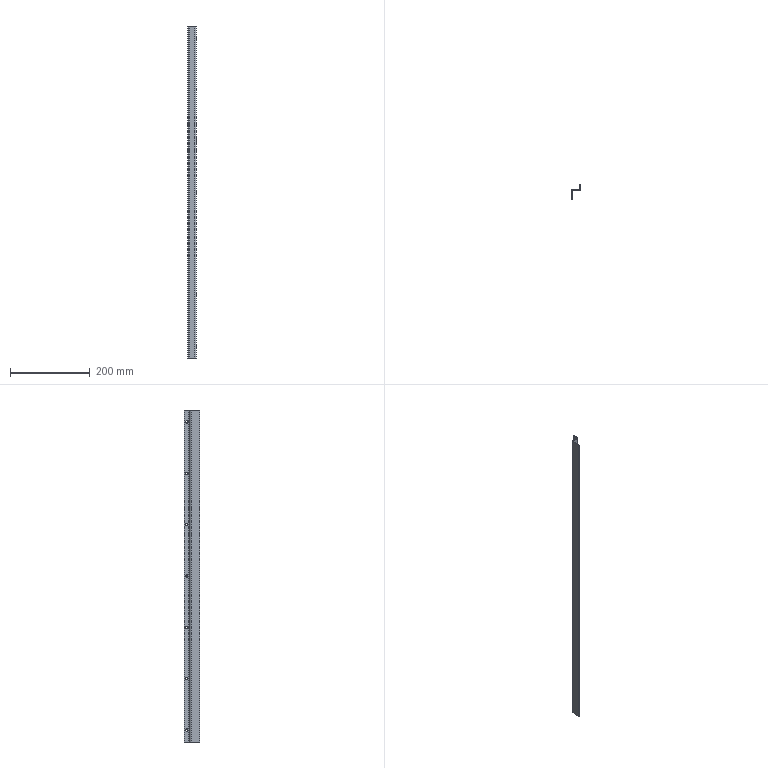Part | NX | features solid 2 | 1 solid | 28 faces | box 22 x 38 x 835 mm | volume 92164 mm3 | cylinder 18 | plane 10 | commonest cylinder face diameters 6 x14 4 x2 8 x2
STEP:
#1=CARTESIAN_POINT('',(1106.,-69.,920.));
#2=VERTEX_POINT('',#1);
#3=CARTESIAN_POINT('',(1108.,-69.,920.));
#4=VERTEX_POINT('',#3);
#5=CARTESIAN_POINT('',(1942.154,-69.,920.));
#6=DIRECTION('',(-1.,0.,0.));
#7=VECTOR('',#6,1000.);
#8=LINE('',#5,#7);
#9=EDGE_CURVE('',#2,#4,#8,.F.);
#10=ORIENTED_EDGE('',*,*,#9,.T.);
#11=CARTESIAN_POINT('',(1108.,-63.,920.));
#12=VERTEX_POINT('',#11);
#13=CARTESIAN_POINT('',(1108.,-66.,920.));
#14=DIRECTION('',(-1.,0.,0.));
#15=DIRECTION('',(0.,1.,0.));
#16=AXIS2_PLACEMENT_3D('',#13,#14,#15);
#17=CIRCLE('',#16,3.);
#18=EDGE_CURVE('',#12,#4,#17,.T.);
#19=ORIENTED_EDGE('',*,*,#18,.F.);
#20=CARTESIAN_POINT('',(1106.,-63.,920.));
#21=VERTEX_POINT('',#20);
#22=CARTESIAN_POINT('',(1942.154,-63.,920.));
#23=DIRECTION('',(-1.,0.,0.));
#24=VECTOR('',#23,1000.);
#25=LINE('',#22,#24);
#26=EDGE_CURVE('',#12,#21,#25,.T.);
#27=ORIENTED_EDGE('',*,*,#26,.T.);
#28=CARTESIAN_POINT('',(1106.,-66.,920.));
#29=DIRECTION('',(-1.,0.,0.));
#30=DIRECTION('',(0.,0.,1.));
#31=AXIS2_PLACEMENT_3D('',#28,#29,#30);
#32=CIRCLE('',#31,3.);
#33=EDGE_CURVE('',#21,#2,#32,.T.);
#34=ORIENTED_EDGE('',*,*,#33,.T.);
#35=EDGE_LOOP('',(#10,#19,#27,#34));
#36=FACE_BOUND('',#35,.T.);
#37=CARTESIAN_POINT('',(1942.154,-66.,920.));
#38=DIRECTION('',(-1.,0.,0.));
#39=DIRECTION('',(0.,1.,0.));
#40=AXIS2_PLACEMENT_3D('',#37,#38,#39);
#41=CYLINDRICAL_SURFACE('',#40,3.);
#42=ADVANCED_FACE('',(#36),#41,.F.);
#43=CARTESIAN_POINT('',(1108.,-69.,790.833));
#44=VERTEX_POINT('',#43);
#45=CARTESIAN_POINT('',(1106.,-69.,790.833));
#46=VERTEX_POINT('',#45);
#47=CARTESIAN_POINT('',(1942.154,-69.,790.833));
#48=DIRECTION('',(-1.,0.,0.));
#49=VECTOR('',#48,1000.);
#50=LINE('',#47,#49);
#51=EDGE_CURVE('',#44,#46,#50,.T.);
#52=ORIENTED_EDGE('',*,*,#51,.F.);
#53=CARTESIAN_POINT('',(1108.,-63.,790.833));
#54=VERTEX_POINT('',#53);
#55=CARTESIAN_POINT('',(1108.,-66.,790.833));
#56=DIRECTION('',(-1.,0.,0.));
#57=DIRECTION('',(0.,1.,0.));
#58=AXIS2_PLACEMENT_3D('',#55,#56,#57);
#59=CIRCLE('',#58,3.);
#60=EDGE_CURVE('',#54,#44,#59,.T.);
#61=ORIENTED_EDGE('',*,*,#60,.F.);
#62=CARTESIAN_POINT('',(1106.,-63.,790.833));
#63=VERTEX_POINT('',#62);
#64=CARTESIAN_POINT('',(1942.154,-63.,790.833));
#65=DIRECTION('',(-1.,0.,0.));
#66=VECTOR('',#65,1000.);
#67=LINE('',#64,#66);
#68=EDGE_CURVE('',#63,#54,#67,.F.);
#69=ORIENTED_EDGE('',*,*,#68,.F.);
#70=CARTESIAN_POINT('',(1106.,-66.,790.833));
#71=DIRECTION('',(-1.,0.,0.));
#72=DIRECTION('',(0.,0.,1.));
#73=AXIS2_PLACEMENT_3D('',#70,#71,#72);
#74=CIRCLE('',#73,3.);
#75=EDGE_CURVE('',#63,#46,#74,.T.);
#76=ORIENTED_EDGE('',*,*,#75,.T.);
#77=EDGE_LOOP('',(#52,#61,#69,#76));
#78=FACE_BOUND('',#77,.T.);
#79=CARTESIAN_POINT('',(1942.154,-66.,790.833));
#80=DIRECTION('',(-1.,0.,0.));
#81=DIRECTION('',(0.,1.,0.));
#82=AXIS2_PLACEMENT_3D('',#79,#80,#81);
#83=CYLINDRICAL_SURFACE('',#82,3.);
#84=ADVANCED_FACE('',(#78),#83,.F.);
#85=CARTESIAN_POINT('',(1108.,-69.,661.667));
#86=VERTEX_POINT('',#85);
#87=CARTESIAN_POINT('',(1106.,-69.,661.667));
#88=VERTEX_POINT('',#87);
#89=CARTESIAN_POINT('',(1942.154,-69.,661.667));
#90=DIRECTION('',(-1.,0.,0.));
#91=VECTOR('',#90,1000.);
#92=LINE('',#89,#91);
#93=EDGE_CURVE('',#86,#88,#92,.T.);
#94=ORIENTED_EDGE('',*,*,#93,.F.);
#95=CARTESIAN_POINT('',(1108.,-63.,661.667));
#96=VERTEX_POINT('',#95);
#97=CARTESIAN_POINT('',(1108.,-66.,661.667));
#98=DIRECTION('',(-1.,0.,0.));
#99=DIRECTION('',(0.,1.,0.));
#100=AXIS2_PLACEMENT_3D('',#97,#98,#99);
#101=CIRCLE('',#100,3.);
#102=EDGE_CURVE('',#96,#86,#101,.T.);
#103=ORIENTED_EDGE('',*,*,#102,.F.);
#104=CARTESIAN_POINT('',(1106.,-63.,661.667));
#105=VERTEX_POINT('',#104);
#106=CARTESIAN_POINT('',(1942.154,-63.,661.667));
#107=DIRECTION('',(-1.,0.,0.));
#108=VECTOR('',#107,1000.);
#109=LINE('',#106,#108);
#110=EDGE_CURVE('',#105,#96,#109,.F.);
#111=ORIENTED_EDGE('',*,*,#110,.F.);
#112=CARTESIAN_POINT('',(1106.,-66.,661.667));
#113=DIRECTION('',(-1.,0.,0.));
#114=DIRECTION('',(0.,0.,1.));
#115=AXIS2_PLACEMENT_3D('',#112,#113,#114);
#116=CIRCLE('',#115,3.);
#117=EDGE_CURVE('',#105,#88,#116,.T.);
#118=ORIENTED_EDGE('',*,*,#117,.T.);
#119=EDGE_LOOP('',(#94,#103,#111,#118));
#120=FACE_BOUND('',#119,.T.);
#121=CARTESIAN_POINT('',(1942.154,-66.,661.667));
#122=DIRECTION('',(-1.,0.,0.));
#123=DIRECTION('',(0.,1.,0.));
#124=AXIS2_PLACEMENT_3D('',#121,#122,#123);
#125=CYLINDRICAL_SURFACE('',#124,3.);
#126=ADVANCED_FACE('',(#120),#125,.F.);
#127=CARTESIAN_POINT('',(1108.,-69.,532.5));
#128=VERTEX_POINT('',#127);
#129=CARTESIAN_POINT('',(1106.,-69.,532.5));
#130=VERTEX_POINT('',#129);
#131=CARTESIAN_POINT('',(1942.154,-69.,532.5));
#132=DIRECTION('',(-1.,0.,0.));
#133=VECTOR('',#132,1000.);
#134=LINE('',#131,#133);
#135=EDGE_CURVE('',#128,#130,#134,.T.);
#136=ORIENTED_EDGE('',*,*,#135,.F.);
#137=CARTESIAN_POINT('',(1108.,-63.,532.5));
#138=VERTEX_POINT('',#137);
#139=CARTESIAN_POINT('',(1108.,-66.,532.5));
#140=DIRECTION('',(-1.,0.,0.));
#141=DIRECTION('',(0.,1.,0.));
#142=AXIS2_PLACEMENT_3D('',#139,#140,#141);
#143=CIRCLE('',#142,3.);
#144=EDGE_CURVE('',#138,#128,#143,.T.);
#145=ORIENTED_EDGE('',*,*,#144,.F.);
#146=CARTESIAN_POINT('',(1106.,-63.,532.5));
#147=VERTEX_POINT('',#146);
#148=CARTESIAN_POINT('',(1942.154,-63.,532.5));
#149=DIRECTION('',(-1.,0.,0.));
#150=VECTOR('',#149,1000.);
#151=LINE('',#148,#150);
#152=EDGE_CURVE('',#147,#138,#151,.F.);
#153=ORIENTED_EDGE('',*,*,#152,.F.);
#154=CARTESIAN_POINT('',(1106.,-66.,532.5));
#155=DIRECTION('',(-1.,0.,0.));
#156=DIRECTION('',(0.,0.,1.));
#157=AXIS2_PLACEMENT_3D('',#154,#155,#156);
#158=CIRCLE('',#157,3.);
#159=EDGE_CURVE('',#147,#130,#158,.T.);
#160=ORIENTED_EDGE('',*,*,#159,.T.);
#161=EDGE_LOOP('',(#136,#145,#153,#160));
#162=FACE_BOUND('',#161,.T.);
#163=CARTESIAN_POINT('',(1942.154,-66.,532.5));
#164=DIRECTION('',(-1.,0.,0.));
#165=DIRECTION('',(0.,1.,0.));
#166=AXIS2_PLACEMENT_3D('',#163,#164,#165);
#167=CYLINDRICAL_SURFACE('',#166,3.);
#168=ADVANCED_FACE('',(#162),#167,.F.);
#169=CARTESIAN_POINT('',(1108.,-69.,403.333));
#170=VERTEX_POINT('',#169);
#171=CARTESIAN_POINT('',(1106.,-69.,403.333));
#172=VERTEX_POINT('',#171);
#173=CARTESIAN_POINT('',(1942.154,-69.,403.333));
#174=DIRECTION('',(-1.,0.,0.));
#175=VECTOR('',#174,1000.);
#176=LINE('',#173,#175);
#177=EDGE_CURVE('',#170,#172,#176,.T.);
#178=ORIENTED_EDGE('',*,*,#177,.F.);
#179=CARTESIAN_POINT('',(1108.,-63.,403.333));
#180=VERTEX_POINT('',#179);
#181=CARTESIAN_POINT('',(1108.,-66.,403.333));
#182=DIRECTION('',(-1.,0.,0.));
#183=DIRECTION('',(0.,1.,0.));
#184=AXIS2_PLACEMENT_3D('',#181,#182,#183);
#185=CIRCLE('',#184,3.);
#186=EDGE_CURVE('',#180,#170,#185,.T.);
#187=ORIENTED_EDGE('',*,*,#186,.F.);
#188=CARTESIAN_POINT('',(1106.,-63.,403.333));
#189=VERTEX_POINT('',#188);
#190=CARTESIAN_POINT('',(1942.154,-63.,403.333));
#191=DIRECTION('',(-1.,0.,0.));
#192=VECTOR('',#191,1000.);
#193=LINE('',#190,#192);
#194=EDGE_CURVE('',#189,#180,#193,.F.);
#195=ORIENTED_EDGE('',*,*,#194,.F.);
#196=CARTESIAN_POINT('',(1106.,-66.,403.333));
#197=DIRECTION('',(-1.,0.,0.));
#198=DIRECTION('',(0.,0.,1.));
#199=AXIS2_PLACEMENT_3D('',#196,#197,#198);
#200=CIRCLE('',#199,3.);
#201=EDGE_CURVE('',#189,#172,#200,.T.);
#202=ORIENTED_EDGE('',*,*,#201,.T.);
#203=EDGE_LOOP('',(#178,#187,#195,#202));
#204=FACE_BOUND('',#203,.T.);
#205=CARTESIAN_POINT('',(1942.154,-66.,403.333));
#206=DIRECTION('',(-1.,0.,0.));
#207=DIRECTION('',(0.,1.,0.));
#208=AXIS2_PLACEMENT_3D('',#205,#206,#207);
#209=CYLINDRICAL_SURFACE('',#208,3.);
#210=ADVANCED_FACE('',(#204),#209,.F.);
#211=CARTESIAN_POINT('',(1106.,-69.,274.167));
#212=VERTEX_POINT('',#211);
#213=CARTESIAN_POINT('',(1108.,-69.,274.167));
#214=VERTEX_POINT('',#213);
#215=CARTESIAN_POINT('',(1942.154,-69.,274.167));
#216=DIRECTION('',(-1.,0.,0.));
#217=VECTOR('',#216,1000.);
#218=LINE('',#215,#217);
#219=EDGE_CURVE('',#212,#214,#218,.F.);
#220=ORIENTED_EDGE('',*,*,#219,.T.);
#221=CARTESIAN_POINT('',(1108.,-63.,274.167));
#222=VERTEX_POINT('',#221);
#223=CARTESIAN_POINT('',(1108.,-66.,274.167));
#224=DIRECTION('',(-1.,0.,0.));
#225=DIRECTION('',(0.,1.,0.));
#226=AXIS2_PLACEMENT_3D('',#223,#224,#225);
#227=CIRCLE('',#226,3.);
#228=EDGE_CURVE('',#222,#214,#227,.T.);
#229=ORIENTED_EDGE('',*,*,#228,.F.);
#230=CARTESIAN_POINT('',(1106.,-63.,274.167));
#231=VERTEX_POINT('',#230);
#232=CARTESIAN_POINT('',(1942.154,-63.,274.167));
#233=DIRECTION('',(-1.,0.,0.));
#234=VECTOR('',#233,1000.);
#235=LINE('',#232,#234);
#236=EDGE_CURVE('',#222,#231,#235,.T.);
#237=ORIENTED_EDGE('',*,*,#236,.T.);
#238=CARTESIAN_POINT('',(1106.,-66.,274.167));
#239=DIRECTION('',(-1.,0.,0.));
#240=DIRECTION('',(0.,0.,1.));
#241=AXIS2_PLACEMENT_3D('',#238,#239,#240);
#242=CIRCLE('',#241,3.);
#243=EDGE_CURVE('',#231,#212,#242,.T.);
#244=ORIENTED_EDGE('',*,*,#243,.T.);
#245=EDGE_LOOP('',(#220,#229,#237,#244));
#246=FACE_BOUND('',#245,.T.);
#247=CARTESIAN_POINT('',(1942.154,-66.,274.167));
#248=DIRECTION('',(-1.,0.,0.));
#249=DIRECTION('',(0.,1.,0.));
#250=AXIS2_PLACEMENT_3D('',#247,#248,#249);
#251=CYLINDRICAL_SURFACE('',#250,3.);
#252=ADVANCED_FACE('',(#246),#251,.F.);
#253=CARTESIAN_POINT('',(1106.,-69.,145.));
#254=VERTEX_POINT('',#253);
#255=CARTESIAN_POINT('',(1108.,-69.,145.));
#256=VERTEX_POINT('',#255);
#257=CARTESIAN_POINT('',(1942.154,-69.,145.));
#258=DIRECTION('',(-1.,0.,0.));
#259=VECTOR('',#258,1000.);
#260=LINE('',#257,#259);
#261=EDGE_CURVE('',#254,#256,#260,.F.);
#262=ORIENTED_EDGE('',*,*,#261,.T.);
#263=CARTESIAN_POINT('',(1108.,-63.,145.));
#264=VERTEX_POINT('',#263);
#265=CARTESIAN_POINT('',(1108.,-66.,145.));
#266=DIRECTION('',(-1.,0.,0.));
#267=DIRECTION('',(0.,1.,0.));
#268=AXIS2_PLACEMENT_3D('',#265,#266,#267);
#269=CIRCLE('',#268,3.);
#270=EDGE_CURVE('',#264,#256,#269,.T.);
#271=ORIENTED_EDGE('',*,*,#270,.F.);
#272=CARTESIAN_POINT('',(1106.,-63.,145.));
#273=VERTEX_POINT('',#272);
#274=CARTESIAN_POINT('',(1942.154,-63.,145.));
#275=DIRECTION('',(-1.,0.,0.));
#276=VECTOR('',#275,1000.);
#277=LINE('',#274,#276);
#278=EDGE_CURVE('',#264,#273,#277,.T.);
#279=ORIENTED_EDGE('',*,*,#278,.T.);
#280=CARTESIAN_POINT('',(1106.,-66.,145.));
#281=DIRECTION('',(-1.,0.,0.));
#282=DIRECTION('',(0.,0.,1.));
#283=AXIS2_PLACEMENT_3D('',#280,#281,#282);
#284=CIRCLE('',#283,3.);
#285=EDGE_CURVE('',#273,#254,#284,.T.);
#286=ORIENTED_EDGE('',*,*,#285,.T.);
#287=EDGE_LOOP('',(#262,#271,#279,#286));
#288=FACE_BOUND('',#287,.T.);
#289=CARTESIAN_POINT('',(1942.154,-66.,145.));
#290=DIRECTION('',(-1.,0.,0.));
#291=DIRECTION('',(0.,1.,0.));
#292=AXIS2_PLACEMENT_3D('',#289,#290,#291);
#293=CYLINDRICAL_SURFACE('',#292,3.);
#294=ADVANCED_FACE('',(#288),#293,.F.);
#295=CARTESIAN_POINT('',(1088.,-77.,950.));
#296=VERTEX_POINT('',#295);
#297=CARTESIAN_POINT('',(1088.,-98.,950.));
#298=VERTEX_POINT('',#297);
#299=CARTESIAN_POINT('',(1088.,-75.,950.));
#300=DIRECTION('',(0.,-1.,0.));
#301=VECTOR('',#300,1000.);
#302=LINE('',#299,#301);
#303=EDGE_CURVE('',#296,#298,#302,.T.);
#304=ORIENTED_EDGE('',*,*,#303,.T.);
#305=CARTESIAN_POINT('',(1088.,-98.,115.));
#306=VERTEX_POINT('',#305);
#307=CARTESIAN_POINT('',(1088.,-98.,115.));
#308=DIRECTION('',(0.,0.,1.));
#309=VECTOR('',#308,1000.);
#310=LINE('',#307,#309);
#311=EDGE_CURVE('',#306,#298,#310,.T.);
#312=ORIENTED_EDGE('',*,*,#311,.F.);
#313=CARTESIAN_POINT('',(1088.,-77.,115.));
#314=VERTEX_POINT('',#313);
#315=CARTESIAN_POINT('',(1088.,-75.,115.));
#316=DIRECTION('',(0.,-1.,0.));
#317=VECTOR('',#316,1000.);
#318=LINE('',#315,#317);
#319=EDGE_CURVE('',#314,#306,#318,.T.);
#320=ORIENTED_EDGE('',*,*,#319,.F.);
#321=CARTESIAN_POINT('',(1088.,-77.,115.));
#322=DIRECTION('',(0.,0.,1.));
#323=VECTOR('',#322,1000.);
#324=LINE('',#321,#323);
#325=EDGE_CURVE('',#314,#296,#324,.T.);
#326=ORIENTED_EDGE('',*,*,#325,.T.);
#327=EDGE_LOOP('',(#304,#312,#320,#326));
#328=FACE_BOUND('',#327,.T.);
#329=CARTESIAN_POINT('',(1088.,-75.,115.));
#330=DIRECTION('',(-1.,0.,0.));
#331=DIRECTION('',(0.,1.,0.));
#332=AXIS2_PLACEMENT_3D('',#329,#330,#331);
#333=PLANE('',#332);
#334=ADVANCED_FACE('',(#328),#333,.F.);
#335=CARTESIAN_POINT('',(1090.,-75.,950.));
#336=VERTEX_POINT('',#335);
#337=CARTESIAN_POINT('',(1090.,-77.,950.));
#338=DIRECTION('',(0.,0.,1.));
#339=DIRECTION('',(0.,1.,0.));
#340=AXIS2_PLACEMENT_3D('',#337,#338,#339);
#341=CIRCLE('',#340,2.);
#342=EDGE_CURVE('',#336,#296,#341,.T.);
#343=ORIENTED_EDGE('',*,*,#342,.T.);
#344=ORIENTED_EDGE('',*,*,#325,.F.);
#345=CARTESIAN_POINT('',(1090.,-75.,115.));
#346=VERTEX_POINT('',#345);
#347=CARTESIAN_POINT('',(1090.,-77.,115.));
#348=DIRECTION('',(0.,0.,1.));
#349=DIRECTION('',(0.,1.,0.));
#350=AXIS2_PLACEMENT_3D('',#347,#348,#349);
#351=CIRCLE('',#350,2.);
#352=EDGE_CURVE('',#346,#314,#351,.T.);
#353=ORIENTED_EDGE('',*,*,#352,.F.);
#354=CARTESIAN_POINT('',(1090.,-75.,115.));
#355=DIRECTION('',(0.,0.,1.));
#356=VECTOR('',#355,1000.);
#357=LINE('',#354,#356);
#358=EDGE_CURVE('',#346,#336,#357,.T.);
#359=ORIENTED_EDGE('',*,*,#358,.T.);
#360=EDGE_LOOP('',(#343,#344,#353,#359));
#361=FACE_BOUND('',#360,.T.);
#362=CARTESIAN_POINT('',(1090.,-77.,115.));
#363=DIRECTION('',(0.,0.,1.));
#364=DIRECTION('',(0.,-1.,0.));
#365=AXIS2_PLACEMENT_3D('',#362,#363,#364);
#366=CYLINDRICAL_SURFACE('',#365,2.);
#367=ADVANCED_FACE('',(#361),#366,.F.);
#368=CARTESIAN_POINT('',(1104.,-75.,950.));
#369=VERTEX_POINT('',#368);
#370=CARTESIAN_POINT('',(1108.,-75.,950.));
#371=DIRECTION('',(-1.,0.,0.));
#372=VECTOR('',#371,1000.);
#373=LINE('',#370,#372);
#374=EDGE_CURVE('',#369,#336,#373,.T.);
#375=ORIENTED_EDGE('',*,*,#374,.T.);
#376=ORIENTED_EDGE('',*,*,#358,.F.);
#377=CARTESIAN_POINT('',(1104.,-75.,115.));
#378=VERTEX_POINT('',#377);
#379=CARTESIAN_POINT('',(1108.,-75.,115.));
#380=DIRECTION('',(-1.,0.,0.));
#381=VECTOR('',#380,1000.);
#382=LINE('',#379,#381);
#383=EDGE_CURVE('',#378,#346,#382,.T.);
#384=ORIENTED_EDGE('',*,*,#383,.F.);
#385=CARTESIAN_POINT('',(1104.,-75.,115.));
#386=DIRECTION('',(0.,0.,1.));
#387=VECTOR('',#386,1000.);
#388=LINE('',#385,#387);
#389=EDGE_CURVE('',#378,#369,#388,.T.);
#390=ORIENTED_EDGE('',*,*,#389,.T.);
#391=EDGE_LOOP('',(#375,#376,#384,#390));
#392=FACE_BOUND('',#391,.T.);
#393=CARTESIAN_POINT('',(1108.,-75.,115.));
#394=DIRECTION('',(0.,1.,0.));
#395=DIRECTION('',(1.,0.,0.));
#396=AXIS2_PLACEMENT_3D('',#393,#394,#395);
#397=PLANE('',#396);
#398=ADVANCED_FACE('',(#392),#397,.F.);
#399=CARTESIAN_POINT('',(1108.,-71.,950.));
#400=VERTEX_POINT('',#399);
#401=CARTESIAN_POINT('',(1104.,-71.,950.));
#402=DIRECTION('',(0.,0.,-1.));
#403=DIRECTION('',(0.,-1.,0.));
#404=AXIS2_PLACEMENT_3D('',#401,#402,#403);
#405=CIRCLE('',#404,4.);
#406=EDGE_CURVE('',#400,#369,#405,.T.);
#407=ORIENTED_EDGE('',*,*,#406,.T.);
#408=ORIENTED_EDGE('',*,*,#389,.F.);
#409=CARTESIAN_POINT('',(1108.,-71.,115.));
#410=VERTEX_POINT('',#409);
#411=CARTESIAN_POINT('',(1104.,-71.,115.));
#412=DIRECTION('',(0.,0.,-1.));
#413=DIRECTION('',(0.,-1.,0.));
#414=AXIS2_PLACEMENT_3D('',#411,#412,#413);
#415=CIRCLE('',#414,4.);
#416=EDGE_CURVE('',#410,#378,#415,.T.);
#417=ORIENTED_EDGE('',*,*,#416,.F.);
#418=CARTESIAN_POINT('',(1108.,-71.,115.));
#419=DIRECTION('',(0.,0.,1.));
#420=VECTOR('',#419,1000.);
#421=LINE('',#418,#420);
#422=EDGE_CURVE('',#410,#400,#421,.T.);
#423=ORIENTED_EDGE('',*,*,#422,.T.);
#424=EDGE_LOOP('',(#407,#408,#417,#423));
#425=FACE_BOUND('',#424,.T.);
#426=CARTESIAN_POINT('',(1104.,-71.,115.));
#427=DIRECTION('',(0.,0.,1.));
#428=DIRECTION('',(0.,-1.,0.));
#429=AXIS2_PLACEMENT_3D('',#426,#427,#428);
#430=CYLINDRICAL_SURFACE('',#429,4.);
#431=ADVANCED_FACE('',(#425),#430,.T.);
#432=ORIENTED_EDGE('',*,*,#270,.T.);
#433=CARTESIAN_POINT('',(1108.,-66.,145.));
#434=DIRECTION('',(-1.,0.,0.));
#435=DIRECTION('',(0.,1.,0.));
#436=AXIS2_PLACEMENT_3D('',#433,#434,#435);
#437=CIRCLE('',#436,3.);
#438=EDGE_CURVE('',#256,#264,#437,.T.);
#439=ORIENTED_EDGE('',*,*,#438,.T.);
#440=EDGE_LOOP('',(#432,#439));
#441=FACE_BOUND('',#440,.T.);
#442=ORIENTED_EDGE('',*,*,#228,.T.);
#443=CARTESIAN_POINT('',(1108.,-66.,274.167));
#444=DIRECTION('',(-1.,0.,0.));
#445=DIRECTION('',(0.,1.,0.));
#446=AXIS2_PLACEMENT_3D('',#443,#444,#445);
#447=CIRCLE('',#446,3.);
#448=EDGE_CURVE('',#214,#222,#447,.T.);
#449=ORIENTED_EDGE('',*,*,#448,.T.);
#450=EDGE_LOOP('',(#442,#449));
#451=FACE_BOUND('',#450,.T.);
#452=ORIENTED_EDGE('',*,*,#186,.T.);
#453=CARTESIAN_POINT('',(1108.,-66.,403.333));
#454=DIRECTION('',(-1.,0.,0.));
#455=DIRECTION('',(0.,1.,0.));
#456=AXIS2_PLACEMENT_3D('',#453,#454,#455);
#457=CIRCLE('',#456,3.);
#458=EDGE_CURVE('',#170,#180,#457,.T.);
#459=ORIENTED_EDGE('',*,*,#458,.T.);
#460=EDGE_LOOP('',(#452,#459));
#461=FACE_BOUND('',#460,.T.);
#462=ORIENTED_EDGE('',*,*,#144,.T.);
#463=CARTESIAN_POINT('',(1108.,-66.,532.5));
#464=DIRECTION('',(-1.,0.,0.));
#465=DIRECTION('',(0.,1.,0.));
#466=AXIS2_PLACEMENT_3D('',#463,#464,#465);
#467=CIRCLE('',#466,3.);
#468=EDGE_CURVE('',#128,#138,#467,.T.);
#469=ORIENTED_EDGE('',*,*,#468,.T.);
#470=EDGE_LOOP('',(#462,#469));
#471=FACE_BOUND('',#470,.T.);
#472=ORIENTED_EDGE('',*,*,#102,.T.);
#473=CARTESIAN_POINT('',(1108.,-66.,661.667));
#474=DIRECTION('',(-1.,0.,0.));
#475=DIRECTION('',(0.,1.,0.));
#476=AXIS2_PLACEMENT_3D('',#473,#474,#475);
#477=CIRCLE('',#476,3.);
#478=EDGE_CURVE('',#86,#96,#477,.T.);
#479=ORIENTED_EDGE('',*,*,#478,.T.);
#480=EDGE_LOOP('',(#472,#479));
#481=FACE_BOUND('',#480,.T.);
#482=ORIENTED_EDGE('',*,*,#60,.T.);
#483=CARTESIAN_POINT('',(1108.,-66.,790.833));
#484=DIRECTION('',(-1.,0.,0.));
#485=DIRECTION('',(0.,1.,0.));
#486=AXIS2_PLACEMENT_3D('',#483,#484,#485);
#487=CIRCLE('',#486,3.);
#488=EDGE_CURVE('',#44,#54,#487,.T.);
#489=ORIENTED_EDGE('',*,*,#488,.T.);
#490=EDGE_LOOP('',(#482,#489));
#491=FACE_BOUND('',#490,.T.);
#492=ORIENTED_EDGE('',*,*,#18,.T.);
#493=CARTESIAN_POINT('',(1108.,-66.,920.));
#494=DIRECTION('',(-1.,0.,0.));
#495=DIRECTION('',(0.,1.,0.));
#496=AXIS2_PLACEMENT_3D('',#493,#494,#495);
#497=CIRCLE('',#496,3.);
#498=EDGE_CURVE('',#4,#12,#497,.T.);
#499=ORIENTED_EDGE('',*,*,#498,.T.);
#500=EDGE_LOOP('',(#492,#499));
#501=FACE_BOUND('',#500,.T.);
#502=CARTESIAN_POINT('',(1108.,-60.,950.));
#503=VERTEX_POINT('',#502);
#504=CARTESIAN_POINT('',(1108.,-60.,950.));
#505=DIRECTION('',(0.,-1.,0.));
#506=VECTOR('',#505,1000.);
#507=LINE('',#504,#506);
#508=EDGE_CURVE('',#503,#400,#507,.T.);
#509=ORIENTED_EDGE('',*,*,#508,.T.);
#510=ORIENTED_EDGE('',*,*,#422,.F.);
#511=CARTESIAN_POINT('',(1108.,-60.,115.));
#512=VERTEX_POINT('',#511);
#513=CARTESIAN_POINT('',(1108.,-60.,115.));
#514=DIRECTION('',(0.,-1.,0.));
#515=VECTOR('',#514,1000.);
#516=LINE('',#513,#515);
#517=EDGE_CURVE('',#512,#410,#516,.T.);
#518=ORIENTED_EDGE('',*,*,#517,.F.);
#519=CARTESIAN_POINT('',(1108.,-60.,115.));
#520=DIRECTION('',(0.,0.,1.));
#521=VECTOR('',#520,1000.);
#522=LINE('',#519,#521);
#523=EDGE_CURVE('',#512,#503,#522,.T.);
#524=ORIENTED_EDGE('',*,*,#523,.T.);
#525=EDGE_LOOP('',(#509,#510,#518,#524));
#526=FACE_BOUND('',#525,.T.);
#527=CARTESIAN_POINT('',(1108.,-60.,115.));
#528=DIRECTION('',(-1.,0.,0.));
#529=DIRECTION('',(0.,1.,0.));
#530=AXIS2_PLACEMENT_3D('',#527,#528,#529);
#531=PLANE('',#530);
#532=ADVANCED_FACE('',(#441,#451,#461,#471,#481,#491,#501,#526),#531,.F.);
#533=CARTESIAN_POINT('',(1086.,-77.,950.));
#534=VERTEX_POINT('',#533);
#535=CARTESIAN_POINT('',(1086.,-98.,950.));
#536=VERTEX_POINT('',#535);
#537=CARTESIAN_POINT('',(1086.,-75.,950.));
#538=DIRECTION('',(0.,-1.,0.));
#539=VECTOR('',#538,1000.);
#540=LINE('',#537,#539);
#541=EDGE_CURVE('',#534,#536,#540,.T.);
#542=ORIENTED_EDGE('',*,*,#541,.F.);
#543=CARTESIAN_POINT('',(1086.,-77.,115.));
#544=VERTEX_POINT('',#543);
#545=CARTESIAN_POINT('',(1086.,-77.,115.));
#546=DIRECTION('',(0.,0.,1.));
#547=VECTOR('',#546,1000.);
#548=LINE('',#545,#547);
#549=EDGE_CURVE('',#544,#534,#548,.T.);
#550=ORIENTED_EDGE('',*,*,#549,.F.);
#551=CARTESIAN_POINT('',(1086.,-98.,115.));
#552=VERTEX_POINT('',#551);
#553=CARTESIAN_POINT('',(1086.,-75.,115.));
#554=DIRECTION('',(0.,-1.,0.));
#555=VECTOR('',#554,1000.);
#556=LINE('',#553,#555);
#557=EDGE_CURVE('',#544,#552,#556,.T.);
#558=ORIENTED_EDGE('',*,*,#557,.T.);
#559=CARTESIAN_POINT('',(1086.,-98.,115.));
#560=DIRECTION('',(0.,0.,1.));
#561=VECTOR('',#560,1000.);
#562=LINE('',#559,#561);
#563=EDGE_CURVE('',#552,#536,#562,.T.);
#564=ORIENTED_EDGE('',*,*,#563,.T.);
#565=EDGE_LOOP('',(#542,#550,#558,#564));
#566=FACE_BOUND('',#565,.T.);
#567=CARTESIAN_POINT('',(1086.,-75.,115.));
#568=DIRECTION('',(-1.,0.,0.));
#569=DIRECTION('',(0.,1.,0.));
#570=AXIS2_PLACEMENT_3D('',#567,#568,#569);
#571=PLANE('',#570);
#572=ADVANCED_FACE('',(#566),#571,.T.);
#573=CARTESIAN_POINT('',(1090.,-73.,950.));
#574=VERTEX_POINT('',#573);
#575=CARTESIAN_POINT('',(1090.,-77.,950.));
#576=DIRECTION('',(0.,0.,1.));
#577=DIRECTION('',(0.,-1.,0.));
#578=AXIS2_PLACEMENT_3D('',#575,#576,#577);
#579=CIRCLE('',#578,4.);
#580=EDGE_CURVE('',#574,#534,#579,.T.);
#581=ORIENTED_EDGE('',*,*,#580,.F.);
#582=CARTESIAN_POINT('',(1090.,-73.,115.));
#583=VERTEX_POINT('',#582);
#584=CARTESIAN_POINT('',(1090.,-73.,115.));
#585=DIRECTION('',(0.,0.,1.));
#586=VECTOR('',#585,1000.);
#587=LINE('',#584,#586);
#588=EDGE_CURVE('',#583,#574,#587,.T.);
#589=ORIENTED_EDGE('',*,*,#588,.F.);
#590=CARTESIAN_POINT('',(1090.,-77.,115.));
#591=DIRECTION('',(0.,0.,1.));
#592=DIRECTION('',(0.,-1.,0.));
#593=AXIS2_PLACEMENT_3D('',#590,#591,#592);
#594=CIRCLE('',#593,4.);
#595=EDGE_CURVE('',#583,#544,#594,.T.);
#596=ORIENTED_EDGE('',*,*,#595,.T.);
#597=ORIENTED_EDGE('',*,*,#549,.T.);
#598=EDGE_LOOP('',(#581,#589,#596,#597));
#599=FACE_BOUND('',#598,.T.);
#600=CARTESIAN_POINT('',(1090.,-77.,115.));
#601=DIRECTION('',(0.,0.,1.));
#602=DIRECTION('',(0.,-1.,0.));
#603=AXIS2_PLACEMENT_3D('',#600,#601,#602);
#604=CYLINDRICAL_SURFACE('',#603,4.);
#605=ADVANCED_FACE('',(#599),#604,.T.);
#606=CARTESIAN_POINT('',(1104.,-73.,950.));
#607=VERTEX_POINT('',#606);
#608=CARTESIAN_POINT('',(1108.,-73.,950.));
#609=DIRECTION('',(-1.,0.,0.));
#610=VECTOR('',#609,1000.);
#611=LINE('',#608,#610);
#612=EDGE_CURVE('',#607,#574,#611,.T.);
#613=ORIENTED_EDGE('',*,*,#612,.F.);
#614=CARTESIAN_POINT('',(1104.,-73.,115.));
#615=VERTEX_POINT('',#614);
#616=CARTESIAN_POINT('',(1104.,-73.,115.));
#617=DIRECTION('',(0.,0.,1.));
#618=VECTOR('',#617,1000.);
#619=LINE('',#616,#618);
#620=EDGE_CURVE('',#615,#607,#619,.T.);
#621=ORIENTED_EDGE('',*,*,#620,.F.);
#622=CARTESIAN_POINT('',(1108.,-73.,115.));
#623=DIRECTION('',(-1.,0.,0.));
#624=VECTOR('',#623,1000.);
#625=LINE('',#622,#624);
#626=EDGE_CURVE('',#615,#583,#625,.T.);
#627=ORIENTED_EDGE('',*,*,#626,.T.);
#628=ORIENTED_EDGE('',*,*,#588,.T.);
#629=EDGE_LOOP('',(#613,#621,#627,#628));
#630=FACE_BOUND('',#629,.T.);
#631=CARTESIAN_POINT('',(1108.,-73.,115.));
#632=DIRECTION('',(0.,1.,0.));
#633=DIRECTION('',(1.,0.,0.));
#634=AXIS2_PLACEMENT_3D('',#631,#632,#633);
#635=PLANE('',#634);
#636=ADVANCED_FACE('',(#630),#635,.T.);
#637=CARTESIAN_POINT('',(1106.,-71.,950.));
#638=VERTEX_POINT('',#637);
#639=CARTESIAN_POINT('',(1104.,-71.,950.));
#640=DIRECTION('',(0.,0.,-1.));
#641=DIRECTION('',(0.,-1.,0.));
#642=AXIS2_PLACEMENT_3D('',#639,#640,#641);
#643=CIRCLE('',#642,2.);
#644=EDGE_CURVE('',#638,#607,#643,.T.);
#645=ORIENTED_EDGE('',*,*,#644,.F.);
#646=CARTESIAN_POINT('',(1106.,-71.,115.));
#647=VERTEX_POINT('',#646);
#648=CARTESIAN_POINT('',(1106.,-71.,115.));
#649=DIRECTION('',(0.,0.,1.));
#650=VECTOR('',#649,1000.);
#651=LINE('',#648,#650);
#652=EDGE_CURVE('',#647,#638,#651,.T.);
#653=ORIENTED_EDGE('',*,*,#652,.F.);
#654=CARTESIAN_POINT('',(1104.,-71.,115.));
#655=DIRECTION('',(0.,0.,-1.));
#656=DIRECTION('',(0.,-1.,0.));
#657=AXIS2_PLACEMENT_3D('',#654,#655,#656);
#658=CIRCLE('',#657,2.);
#659=EDGE_CURVE('',#647,#615,#658,.T.);
#660=ORIENTED_EDGE('',*,*,#659,.T.);
#661=ORIENTED_EDGE('',*,*,#620,.T.);
#662=EDGE_LOOP('',(#645,#653,#660,#661));
#663=FACE_BOUND('',#662,.T.);
#664=CARTESIAN_POINT('',(1104.,-71.,115.));
#665=DIRECTION('',(0.,0.,1.));
#666=DIRECTION('',(0.,-1.,0.));
#667=AXIS2_PLACEMENT_3D('',#664,#665,#666);
#668=CYLINDRICAL_SURFACE('',#667,2.);
#669=ADVANCED_FACE('',(#663),#668,.F.);
#670=ORIENTED_EDGE('',*,*,#285,.F.);
#671=CARTESIAN_POINT('',(1106.,-66.,145.));
#672=DIRECTION('',(-1.,0.,0.));
#673=DIRECTION('',(0.,0.,1.));
#674=AXIS2_PLACEMENT_3D('',#671,#672,#673);
#675=CIRCLE('',#674,3.);
#676=EDGE_CURVE('',#254,#273,#675,.T.);
#677=ORIENTED_EDGE('',*,*,#676,.F.);
#678=EDGE_LOOP('',(#670,#677));
#679=FACE_BOUND('',#678,.T.);
#680=ORIENTED_EDGE('',*,*,#243,.F.);
#681=CARTESIAN_POINT('',(1106.,-66.,274.167));
#682=DIRECTION('',(-1.,0.,0.));
#683=DIRECTION('',(0.,0.,1.));
#684=AXIS2_PLACEMENT_3D('',#681,#682,#683);
#685=CIRCLE('',#684,3.);
#686=EDGE_CURVE('',#212,#231,#685,.T.);
#687=ORIENTED_EDGE('',*,*,#686,.F.);
#688=EDGE_LOOP('',(#680,#687));
#689=FACE_BOUND('',#688,.T.);
#690=ORIENTED_EDGE('',*,*,#201,.F.);
#691=CARTESIAN_POINT('',(1106.,-66.,403.333));
#692=DIRECTION('',(-1.,0.,0.));
#693=DIRECTION('',(0.,0.,1.));
#694=AXIS2_PLACEMENT_3D('',#691,#692,#693);
#695=CIRCLE('',#694,3.);
#696=EDGE_CURVE('',#172,#189,#695,.T.);
#697=ORIENTED_EDGE('',*,*,#696,.F.);
#698=EDGE_LOOP('',(#690,#697));
#699=FACE_BOUND('',#698,.T.);
#700=ORIENTED_EDGE('',*,*,#159,.F.);
#701=CARTESIAN_POINT('',(1106.,-66.,532.5));
#702=DIRECTION('',(-1.,0.,0.));
#703=DIRECTION('',(0.,0.,1.));
#704=AXIS2_PLACEMENT_3D('',#701,#702,#703);
#705=CIRCLE('',#704,3.);
#706=EDGE_CURVE('',#130,#147,#705,.T.);
#707=ORIENTED_EDGE('',*,*,#706,.F.);
#708=EDGE_LOOP('',(#700,#707));
#709=FACE_BOUND('',#708,.T.);
#710=ORIENTED_EDGE('',*,*,#117,.F.);
#711=CARTESIAN_POINT('',(1106.,-66.,661.667));
#712=DIRECTION('',(-1.,0.,0.));
#713=DIRECTION('',(0.,0.,1.));
#714=AXIS2_PLACEMENT_3D('',#711,#712,#713);
#715=CIRCLE('',#714,3.);
#716=EDGE_CURVE('',#88,#105,#715,.T.);
#717=ORIENTED_EDGE('',*,*,#716,.F.);
#718=EDGE_LOOP('',(#710,#717));
#719=FACE_BOUND('',#718,.T.);
#720=ORIENTED_EDGE('',*,*,#75,.F.);
#721=CARTESIAN_POINT('',(1106.,-66.,790.833));
#722=DIRECTION('',(-1.,0.,0.));
#723=DIRECTION('',(0.,0.,1.));
#724=AXIS2_PLACEMENT_3D('',#721,#722,#723);
#725=CIRCLE('',#724,3.);
#726=EDGE_CURVE('',#46,#63,#725,.T.);
#727=ORIENTED_EDGE('',*,*,#726,.F.);
#728=EDGE_LOOP('',(#720,#727));
#729=FACE_BOUND('',#728,.T.);
#730=ORIENTED_EDGE('',*,*,#33,.F.);
#731=CARTESIAN_POINT('',(1106.,-66.,920.));
#732=DIRECTION('',(-1.,0.,0.));
#733=DIRECTION('',(0.,0.,1.));
#734=AXIS2_PLACEMENT_3D('',#731,#732,#733);
#735=CIRCLE('',#734,3.);
#736=EDGE_CURVE('',#2,#21,#735,.T.);
#737=ORIENTED_EDGE('',*,*,#736,.F.);
#738=EDGE_LOOP('',(#730,#737));
#739=FACE_BOUND('',#738,.T.);
#740=CARTESIAN_POINT('',(1106.,-60.,950.));
#741=VERTEX_POINT('',#740);
#742=CARTESIAN_POINT('',(1106.,-60.,950.));
#743=DIRECTION('',(0.,-1.,0.));
#744=VECTOR('',#743,1000.);
#745=LINE('',#742,#744);
#746=EDGE_CURVE('',#741,#638,#745,.T.);
#747=ORIENTED_EDGE('',*,*,#746,.F.);
#748=CARTESIAN_POINT('',(1106.,-60.,115.));
#749=VERTEX_POINT('',#748);
#750=CARTESIAN_POINT('',(1106.,-60.,115.));
#751=DIRECTION('',(0.,0.,1.));
#752=VECTOR('',#751,1000.);
#753=LINE('',#750,#752);
#754=EDGE_CURVE('',#749,#741,#753,.T.);
#755=ORIENTED_EDGE('',*,*,#754,.F.);
#756=CARTESIAN_POINT('',(1106.,-60.,115.));
#757=DIRECTION('',(0.,-1.,0.));
#758=VECTOR('',#757,1000.);
#759=LINE('',#756,#758);
#760=EDGE_CURVE('',#749,#647,#759,.T.);
#761=ORIENTED_EDGE('',*,*,#760,.T.);
#762=ORIENTED_EDGE('',*,*,#652,.T.);
#763=EDGE_LOOP('',(#747,#755,#761,#762));
#764=FACE_BOUND('',#763,.T.);
#765=CARTESIAN_POINT('',(1106.,-60.,115.));
#766=DIRECTION('',(-1.,0.,0.));
#767=DIRECTION('',(0.,1.,0.));
#768=AXIS2_PLACEMENT_3D('',#765,#766,#767);
#769=PLANE('',#768);
#770=ADVANCED_FACE('',(#679,#689,#699,#709,#719,#729,#739,#764),#769,.T.);
#771=ORIENTED_EDGE('',*,*,#523,.F.);
#772=CARTESIAN_POINT('',(1108.,-60.,115.));
#773=DIRECTION('',(-1.,0.,0.));
#774=VECTOR('',#773,1000.);
#775=LINE('',#772,#774);
#776=EDGE_CURVE('',#512,#749,#775,.T.);
#777=ORIENTED_EDGE('',*,*,#776,.T.);
#778=ORIENTED_EDGE('',*,*,#754,.T.);
#779=CARTESIAN_POINT('',(1108.,-60.,950.));
#780=DIRECTION('',(-1.,0.,0.));
#781=VECTOR('',#780,1000.);
#782=LINE('',#779,#781);
#783=EDGE_CURVE('',#503,#741,#782,.T.);
#784=ORIENTED_EDGE('',*,*,#783,.F.);
#785=EDGE_LOOP('',(#771,#777,#778,#784));
#786=FACE_BOUND('',#785,.T.);
#787=CARTESIAN_POINT('',(1108.,-60.,115.));
#788=DIRECTION('',(0.,-1.,0.));
#789=DIRECTION('',(0.,0.,-1.));
#790=AXIS2_PLACEMENT_3D('',#787,#788,#789);
#791=PLANE('',#790);
#792=ADVANCED_FACE('',(#786),#791,.F.);
#793=ORIENTED_EDGE('',*,*,#746,.T.);
#794=ORIENTED_EDGE('',*,*,#644,.T.);
#795=ORIENTED_EDGE('',*,*,#612,.T.);
#796=ORIENTED_EDGE('',*,*,#580,.T.);
#797=ORIENTED_EDGE('',*,*,#541,.T.);
#798=CARTESIAN_POINT('',(1088.,-98.,950.));
#799=DIRECTION('',(-1.,0.,0.));
#800=VECTOR('',#799,1000.);
#801=LINE('',#798,#800);
#802=EDGE_CURVE('',#298,#536,#801,.T.);
#803=ORIENTED_EDGE('',*,*,#802,.F.);
#804=ORIENTED_EDGE('',*,*,#303,.F.);
#805=ORIENTED_EDGE('',*,*,#342,.F.);
#806=ORIENTED_EDGE('',*,*,#374,.F.);
#807=ORIENTED_EDGE('',*,*,#406,.F.);
#808=ORIENTED_EDGE('',*,*,#508,.F.);
#809=ORIENTED_EDGE('',*,*,#783,.T.);
#810=EDGE_LOOP('',(#793,#794,#795,#796,#797,#803,#804,#805,#806,#807,#808,#809));
#811=FACE_BOUND('',#810,.T.);
#812=CARTESIAN_POINT('',(1108.,-60.,950.));
#813=DIRECTION('',(0.,0.,-1.));
#814=DIRECTION('',(0.,-1.,0.));
#815=AXIS2_PLACEMENT_3D('',#812,#813,#814);
#816=PLANE('',#815);
#817=ADVANCED_FACE('',(#811),#816,.F.);
#818=CARTESIAN_POINT('',(1088.,-98.,115.));
#819=DIRECTION('',(-1.,0.,0.));
#820=VECTOR('',#819,1000.);
#821=LINE('',#818,#820);
#822=EDGE_CURVE('',#306,#552,#821,.T.);
#823=ORIENTED_EDGE('',*,*,#822,.F.);
#824=ORIENTED_EDGE('',*,*,#311,.T.);
#825=ORIENTED_EDGE('',*,*,#802,.T.);
#826=ORIENTED_EDGE('',*,*,#563,.F.);
#827=EDGE_LOOP('',(#823,#824,#825,#826));
#828=FACE_BOUND('',#827,.T.);
#829=CARTESIAN_POINT('',(1088.,-98.,115.));
#830=DIRECTION('',(0.,-1.,0.));
#831=DIRECTION('',(0.,0.,-1.));
#832=AXIS2_PLACEMENT_3D('',#829,#830,#831);
#833=PLANE('',#832);
#834=ADVANCED_FACE('',(#828),#833,.T.);
#835=ORIENTED_EDGE('',*,*,#557,.F.);
#836=ORIENTED_EDGE('',*,*,#595,.F.);
#837=ORIENTED_EDGE('',*,*,#626,.F.);
#838=ORIENTED_EDGE('',*,*,#659,.F.);
#839=ORIENTED_EDGE('',*,*,#760,.F.);
#840=ORIENTED_EDGE('',*,*,#776,.F.);
#841=ORIENTED_EDGE('',*,*,#517,.T.);
#842=ORIENTED_EDGE('',*,*,#416,.T.);
#843=ORIENTED_EDGE('',*,*,#383,.T.);
#844=ORIENTED_EDGE('',*,*,#352,.T.);
#845=ORIENTED_EDGE('',*,*,#319,.T.);
#846=ORIENTED_EDGE('',*,*,#822,.T.);
#847=EDGE_LOOP('',(#835,#836,#837,#838,#839,#840,#841,#842,#843,#844,#845,#846));
#848=FACE_BOUND('',#847,.T.);
#849=CARTESIAN_POINT('',(1088.,-75.,115.));
#850=DIRECTION('',(0.,0.,-1.));
#851=DIRECTION('',(0.,-1.,0.));
#852=AXIS2_PLACEMENT_3D('',#849,#850,#851);
#853=PLANE('',#852);
#854=ADVANCED_FACE('',(#848),#853,.T.);
#855=ORIENTED_EDGE('',*,*,#438,.F.);
#856=ORIENTED_EDGE('',*,*,#261,.F.);
#857=ORIENTED_EDGE('',*,*,#676,.T.);
#858=ORIENTED_EDGE('',*,*,#278,.F.);
#859=EDGE_LOOP('',(#855,#856,#857,#858));
#860=FACE_BOUND('',#859,.T.);
#861=CARTESIAN_POINT('',(1942.154,-66.,145.));
#862=DIRECTION('',(-1.,0.,0.));
#863=DIRECTION('',(0.,1.,0.));
#864=AXIS2_PLACEMENT_3D('',#861,#862,#863);
#865=CYLINDRICAL_SURFACE('',#864,3.);
#866=ADVANCED_FACE('',(#860),#865,.F.);
#867=ORIENTED_EDGE('',*,*,#448,.F.);
#868=ORIENTED_EDGE('',*,*,#219,.F.);
#869=ORIENTED_EDGE('',*,*,#686,.T.);
#870=ORIENTED_EDGE('',*,*,#236,.F.);
#871=EDGE_LOOP('',(#867,#868,#869,#870));
#872=FACE_BOUND('',#871,.T.);
#873=CARTESIAN_POINT('',(1942.154,-66.,274.167));
#874=DIRECTION('',(-1.,0.,0.));
#875=DIRECTION('',(0.,1.,0.));
#876=AXIS2_PLACEMENT_3D('',#873,#874,#875);
#877=CYLINDRICAL_SURFACE('',#876,3.);
#878=ADVANCED_FACE('',(#872),#877,.F.);
#879=ORIENTED_EDGE('',*,*,#458,.F.);
#880=ORIENTED_EDGE('',*,*,#177,.T.);
#881=ORIENTED_EDGE('',*,*,#696,.T.);
#882=ORIENTED_EDGE('',*,*,#194,.T.);
#883=EDGE_LOOP('',(#879,#880,#881,#882));
#884=FACE_BOUND('',#883,.T.);
#885=CARTESIAN_POINT('',(1942.154,-66.,403.333));
#886=DIRECTION('',(-1.,0.,0.));
#887=DIRECTION('',(0.,1.,0.));
#888=AXIS2_PLACEMENT_3D('',#885,#886,#887);
#889=CYLINDRICAL_SURFACE('',#888,3.);
#890=ADVANCED_FACE('',(#884),#889,.F.);
#891=ORIENTED_EDGE('',*,*,#468,.F.);
#892=ORIENTED_EDGE('',*,*,#135,.T.);
#893=ORIENTED_EDGE('',*,*,#706,.T.);
#894=ORIENTED_EDGE('',*,*,#152,.T.);
#895=EDGE_LOOP('',(#891,#892,#893,#894));
#896=FACE_BOUND('',#895,.T.);
#897=CARTESIAN_POINT('',(1942.154,-66.,532.5));
#898=DIRECTION('',(-1.,0.,0.));
#899=DIRECTION('',(0.,1.,0.));
#900=AXIS2_PLACEMENT_3D('',#897,#898,#899);
#901=CYLINDRICAL_SURFACE('',#900,3.);
#902=ADVANCED_FACE('',(#896),#901,.F.);
#903=ORIENTED_EDGE('',*,*,#478,.F.);
#904=ORIENTED_EDGE('',*,*,#93,.T.);
#905=ORIENTED_EDGE('',*,*,#716,.T.);
#906=ORIENTED_EDGE('',*,*,#110,.T.);
#907=EDGE_LOOP('',(#903,#904,#905,#906));
#908=FACE_BOUND('',#907,.T.);
#909=CARTESIAN_POINT('',(1942.154,-66.,661.667));
#910=DIRECTION('',(-1.,0.,0.));
#911=DIRECTION('',(0.,1.,0.));
#912=AXIS2_PLACEMENT_3D('',#909,#910,#911);
#913=CYLINDRICAL_SURFACE('',#912,3.);
#914=ADVANCED_FACE('',(#908),#913,.F.);
#915=ORIENTED_EDGE('',*,*,#488,.F.);
#916=ORIENTED_EDGE('',*,*,#51,.T.);
#917=ORIENTED_EDGE('',*,*,#726,.T.);
#918=ORIENTED_EDGE('',*,*,#68,.T.);
#919=EDGE_LOOP('',(#915,#916,#917,#918));
#920=FACE_BOUND('',#919,.T.);
#921=CARTESIAN_POINT('',(1942.154,-66.,790.833));
#922=DIRECTION('',(-1.,0.,0.));
#923=DIRECTION('',(0.,1.,0.));
#924=AXIS2_PLACEMENT_3D('',#921,#922,#923);
#925=CYLINDRICAL_SURFACE('',#924,3.);
#926=ADVANCED_FACE('',(#920),#925,.F.);
#927=ORIENTED_EDGE('',*,*,#498,.F.);
#928=ORIENTED_EDGE('',*,*,#9,.F.);
#929=ORIENTED_EDGE('',*,*,#736,.T.);
#930=ORIENTED_EDGE('',*,*,#26,.F.);
#931=EDGE_LOOP('',(#927,#928,#929,#930));
#932=FACE_BOUND('',#931,.T.);
#933=CARTESIAN_POINT('',(1942.154,-66.,920.));
#934=DIRECTION('',(-1.,0.,0.));
#935=DIRECTION('',(0.,1.,0.));
#936=AXIS2_PLACEMENT_3D('',#933,#934,#935);
#937=CYLINDRICAL_SURFACE('',#936,3.);
#938=ADVANCED_FACE('',(#932),#937,.F.);
#939=CLOSED_SHELL('',(#42,#84,#126,#168,#210,#252,#294,#334,#367,#398,#431,#532,#572,#605,#636,#669,#770,#792,#817,#834,#854,#866,#878,#890,#902,#914,#926,#938));
#940=MANIFOLD_SOLID_BREP('',#939);
#941=(LENGTH_UNIT()NAMED_UNIT(*)SI_UNIT(.MILLI.,.METRE.));
#942=UNCERTAINTY_MEASURE_WITH_UNIT(LENGTH_MEASURE(0.00001),#941,'','');
#943=(NAMED_UNIT(*)PLANE_ANGLE_UNIT()SI_UNIT($,.RADIAN.));
#944=(NAMED_UNIT(*)SI_UNIT($,.STERADIAN.)SOLID_ANGLE_UNIT());
#945=(GEOMETRIC_REPRESENTATION_CONTEXT(3)GLOBAL_UNCERTAINTY_ASSIGNED_CONTEXT((#942))GLOBAL_UNIT_ASSIGNED_CONTEXT((#941,#943,#944))REPRESENTATION_CONTEXT('',''));
#946=ADVANCED_BREP_SHAPE_REPRESENTATION('',(#940),#945);